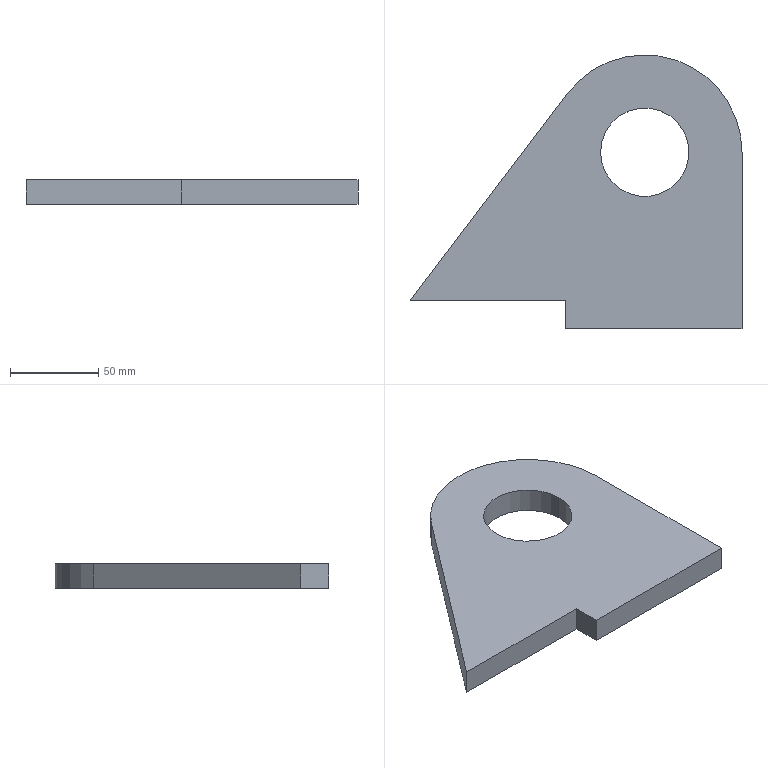Part | SolidWorks | features Extrusion 1, ICE 1 | 1 solid | 10 faces | box 187.85 x 155 x 14 mm | volume 247165 mm3 | plane 7 | cylinder 3 | commonest cylinder face diameters 50 x2 110 x1
STEP:
#1=CARTESIAN_POINT('',(-25.,0.,14.));
#2=VERTEX_POINT('',#1);
#3=CARTESIAN_POINT('',(25.,0.,14.));
#4=VERTEX_POINT('',#3);
#5=CARTESIAN_POINT('',(0.,0.,14.));
#6=DIRECTION('',(0.,0.,1.));
#7=DIRECTION('',(1.,0.,0.));
#8=AXIS2_PLACEMENT_3D('',#5,#6,#7);
#9=CIRCLE('',#8,25.);
#10=EDGE_CURVE('',#2,#4,#9,.T.);
#11=ORIENTED_EDGE('',*,*,#10,.T.);
#12=CARTESIAN_POINT('',(25.,0.,0.));
#13=VERTEX_POINT('',#12);
#14=CARTESIAN_POINT('',(25.,0.,14.));
#15=DIRECTION('',(0.,0.,-1.));
#16=VECTOR('',#15,1000.);
#17=LINE('',#14,#16);
#18=EDGE_CURVE('',#4,#13,#17,.T.);
#19=ORIENTED_EDGE('',*,*,#18,.T.);
#20=CARTESIAN_POINT('',(-25.,0.,0.));
#21=VERTEX_POINT('',#20);
#22=CARTESIAN_POINT('',(0.,0.,0.));
#23=DIRECTION('',(0.,0.,1.));
#24=DIRECTION('',(1.,0.,0.));
#25=AXIS2_PLACEMENT_3D('',#22,#23,#24);
#26=CIRCLE('',#25,25.);
#27=EDGE_CURVE('',#21,#13,#26,.T.);
#28=ORIENTED_EDGE('',*,*,#27,.F.);
#29=CARTESIAN_POINT('',(-25.,0.,14.));
#30=DIRECTION('',(0.,0.,-1.));
#31=VECTOR('',#30,1000.);
#32=LINE('',#29,#31);
#33=EDGE_CURVE('',#2,#21,#32,.T.);
#34=ORIENTED_EDGE('',*,*,#33,.F.);
#35=EDGE_LOOP('',(#11,#19,#28,#34));
#36=FACE_OUTER_BOUND('',#35,.T.);
#37=CARTESIAN_POINT('',(0.,0.,14.));
#38=DIRECTION('',(0.,0.,-1.));
#39=DIRECTION('',(-1.,0.,0.));
#40=AXIS2_PLACEMENT_3D('',#37,#38,#39);
#41=CYLINDRICAL_SURFACE('',#40,25.);
#42=ADVANCED_FACE('',(#36),#41,.F.);
#43=CARTESIAN_POINT('',(-45.,-84.,14.));
#44=VERTEX_POINT('',#43);
#45=CARTESIAN_POINT('',(-132.85,-84.,14.));
#46=VERTEX_POINT('',#45);
#47=CARTESIAN_POINT('',(-145.,-84.,14.));
#48=DIRECTION('',(-1.,0.,0.));
#49=VECTOR('',#48,1000.);
#50=LINE('',#47,#49);
#51=EDGE_CURVE('',#44,#46,#50,.T.);
#52=ORIENTED_EDGE('',*,*,#51,.F.);
#53=CARTESIAN_POINT('',(-45.,-100.,14.));
#54=VERTEX_POINT('',#53);
#55=CARTESIAN_POINT('',(-45.,-100.,14.));
#56=DIRECTION('',(0.,1.,0.));
#57=VECTOR('',#56,1000.);
#58=LINE('',#55,#57);
#59=EDGE_CURVE('',#54,#44,#58,.T.);
#60=ORIENTED_EDGE('',*,*,#59,.F.);
#61=CARTESIAN_POINT('',(55.,-100.,14.));
#62=VERTEX_POINT('',#61);
#63=CARTESIAN_POINT('',(-145.,-100.,14.));
#64=DIRECTION('',(1.,0.,0.));
#65=VECTOR('',#64,1000.);
#66=LINE('',#63,#65);
#67=EDGE_CURVE('',#54,#62,#66,.T.);
#68=ORIENTED_EDGE('',*,*,#67,.T.);
#69=CARTESIAN_POINT('',(55.,0.,14.));
#70=VERTEX_POINT('',#69);
#71=CARTESIAN_POINT('',(55.,0.,14.));
#72=DIRECTION('',(0.,1.,0.));
#73=VECTOR('',#72,1000.);
#74=LINE('',#71,#73);
#75=EDGE_CURVE('',#62,#70,#74,.T.);
#76=ORIENTED_EDGE('',*,*,#75,.T.);
#77=CARTESIAN_POINT('',(-43.802,33.263,14.));
#78=VERTEX_POINT('',#77);
#79=CARTESIAN_POINT('',(0.,0.,14.));
#80=DIRECTION('',(0.,0.,1.));
#81=DIRECTION('',(1.,0.,0.));
#82=AXIS2_PLACEMENT_3D('',#79,#80,#81);
#83=CIRCLE('',#82,55.);
#84=EDGE_CURVE('',#70,#78,#83,.T.);
#85=ORIENTED_EDGE('',*,*,#84,.T.);
#86=CARTESIAN_POINT('',(-43.802,33.263,14.));
#87=DIRECTION('',(-0.6048,-0.7964,0.));
#88=VECTOR('',#87,1000.);
#89=LINE('',#86,#88);
#90=EDGE_CURVE('',#78,#46,#89,.T.);
#91=ORIENTED_EDGE('',*,*,#90,.T.);
#92=EDGE_LOOP('',(#52,#60,#68,#76,#85,#91));
#93=FACE_OUTER_BOUND('',#92,.T.);
#94=ORIENTED_EDGE('',*,*,#10,.F.);
#95=CARTESIAN_POINT('',(0.,0.,14.));
#96=DIRECTION('',(0.,0.,1.));
#97=DIRECTION('',(1.,0.,0.));
#98=AXIS2_PLACEMENT_3D('',#95,#96,#97);
#99=CIRCLE('',#98,25.);
#100=EDGE_CURVE('',#4,#2,#99,.T.);
#101=ORIENTED_EDGE('',*,*,#100,.F.);
#102=EDGE_LOOP('',(#94,#101));
#103=FACE_BOUND('',#102,.T.);
#104=CARTESIAN_POINT('',(0.,0.,14.));
#105=DIRECTION('',(0.,0.,1.));
#106=DIRECTION('',(1.,0.,0.));
#107=AXIS2_PLACEMENT_3D('',#104,#105,#106);
#108=PLANE('',#107);
#109=ADVANCED_FACE('',(#93,#103),#108,.T.);
#110=CARTESIAN_POINT('',(-45.,-100.,0.));
#111=VERTEX_POINT('',#110);
#112=CARTESIAN_POINT('',(-45.,-84.,0.));
#113=VERTEX_POINT('',#112);
#114=CARTESIAN_POINT('',(-45.,-100.,0.));
#115=DIRECTION('',(0.,1.,0.));
#116=VECTOR('',#115,1000.);
#117=LINE('',#114,#116);
#118=EDGE_CURVE('',#111,#113,#117,.T.);
#119=ORIENTED_EDGE('',*,*,#118,.T.);
#120=CARTESIAN_POINT('',(-132.85,-84.,0.));
#121=VERTEX_POINT('',#120);
#122=CARTESIAN_POINT('',(-145.,-84.,0.));
#123=DIRECTION('',(-1.,0.,0.));
#124=VECTOR('',#123,1000.);
#125=LINE('',#122,#124);
#126=EDGE_CURVE('',#113,#121,#125,.T.);
#127=ORIENTED_EDGE('',*,*,#126,.T.);
#128=CARTESIAN_POINT('',(-43.802,33.263,0.));
#129=VERTEX_POINT('',#128);
#130=CARTESIAN_POINT('',(-43.802,33.263,0.));
#131=DIRECTION('',(-0.6048,-0.7964,0.));
#132=VECTOR('',#131,1000.);
#133=LINE('',#130,#132);
#134=EDGE_CURVE('',#129,#121,#133,.T.);
#135=ORIENTED_EDGE('',*,*,#134,.F.);
#136=CARTESIAN_POINT('',(55.,0.,0.));
#137=VERTEX_POINT('',#136);
#138=CARTESIAN_POINT('',(0.,0.,0.));
#139=DIRECTION('',(0.,0.,1.));
#140=DIRECTION('',(1.,0.,0.));
#141=AXIS2_PLACEMENT_3D('',#138,#139,#140);
#142=CIRCLE('',#141,55.);
#143=EDGE_CURVE('',#137,#129,#142,.T.);
#144=ORIENTED_EDGE('',*,*,#143,.F.);
#145=CARTESIAN_POINT('',(55.,-100.,0.));
#146=VERTEX_POINT('',#145);
#147=CARTESIAN_POINT('',(55.,0.,0.));
#148=DIRECTION('',(0.,1.,0.));
#149=VECTOR('',#148,1000.);
#150=LINE('',#147,#149);
#151=EDGE_CURVE('',#146,#137,#150,.T.);
#152=ORIENTED_EDGE('',*,*,#151,.F.);
#153=CARTESIAN_POINT('',(-145.,-100.,0.));
#154=DIRECTION('',(1.,0.,0.));
#155=VECTOR('',#154,1000.);
#156=LINE('',#153,#155);
#157=EDGE_CURVE('',#111,#146,#156,.T.);
#158=ORIENTED_EDGE('',*,*,#157,.F.);
#159=EDGE_LOOP('',(#119,#127,#135,#144,#152,#158));
#160=FACE_OUTER_BOUND('',#159,.T.);
#161=ORIENTED_EDGE('',*,*,#27,.T.);
#162=CARTESIAN_POINT('',(0.,0.,0.));
#163=DIRECTION('',(0.,0.,1.));
#164=DIRECTION('',(1.,0.,0.));
#165=AXIS2_PLACEMENT_3D('',#162,#163,#164);
#166=CIRCLE('',#165,25.);
#167=EDGE_CURVE('',#13,#21,#166,.T.);
#168=ORIENTED_EDGE('',*,*,#167,.T.);
#169=EDGE_LOOP('',(#161,#168));
#170=FACE_BOUND('',#169,.T.);
#171=CARTESIAN_POINT('',(0.,0.,0.));
#172=DIRECTION('',(0.,0.,1.));
#173=DIRECTION('',(1.,0.,0.));
#174=AXIS2_PLACEMENT_3D('',#171,#172,#173);
#175=PLANE('',#174);
#176=ADVANCED_FACE('',(#160,#170),#175,.F.);
#177=ORIENTED_EDGE('',*,*,#143,.T.);
#178=CARTESIAN_POINT('',(-43.802,33.263,14.));
#179=DIRECTION('',(0.,0.,-1.));
#180=VECTOR('',#179,1000.);
#181=LINE('',#178,#180);
#182=EDGE_CURVE('',#78,#129,#181,.T.);
#183=ORIENTED_EDGE('',*,*,#182,.F.);
#184=ORIENTED_EDGE('',*,*,#84,.F.);
#185=CARTESIAN_POINT('',(55.,0.,14.));
#186=DIRECTION('',(0.,0.,-1.));
#187=VECTOR('',#186,1000.);
#188=LINE('',#185,#187);
#189=EDGE_CURVE('',#70,#137,#188,.T.);
#190=ORIENTED_EDGE('',*,*,#189,.T.);
#191=EDGE_LOOP('',(#177,#183,#184,#190));
#192=FACE_OUTER_BOUND('',#191,.T.);
#193=CARTESIAN_POINT('',(0.,0.,14.));
#194=DIRECTION('',(0.,0.,-1.));
#195=DIRECTION('',(-1.,0.,0.));
#196=AXIS2_PLACEMENT_3D('',#193,#194,#195);
#197=CYLINDRICAL_SURFACE('',#196,55.);
#198=ADVANCED_FACE('',(#192),#197,.T.);
#199=ORIENTED_EDGE('',*,*,#134,.T.);
#200=CARTESIAN_POINT('',(-132.85,-84.,14.));
#201=DIRECTION('',(0.,0.,1.));
#202=VECTOR('',#201,1000.);
#203=LINE('',#200,#202);
#204=EDGE_CURVE('',#121,#46,#203,.T.);
#205=ORIENTED_EDGE('',*,*,#204,.T.);
#206=ORIENTED_EDGE('',*,*,#90,.F.);
#207=ORIENTED_EDGE('',*,*,#182,.T.);
#208=EDGE_LOOP('',(#199,#205,#206,#207));
#209=FACE_OUTER_BOUND('',#208,.T.);
#210=CARTESIAN_POINT('',(-43.802,33.263,14.));
#211=DIRECTION('',(0.7964,-0.6048,0.));
#212=DIRECTION('',(0.6048,0.7964,0.));
#213=AXIS2_PLACEMENT_3D('',#210,#211,#212);
#214=PLANE('',#213);
#215=ADVANCED_FACE('',(#209),#214,.F.);
#216=ORIENTED_EDGE('',*,*,#67,.F.);
#217=CARTESIAN_POINT('',(-45.,-100.,0.));
#218=DIRECTION('',(0.,0.,1.));
#219=VECTOR('',#218,1000.);
#220=LINE('',#217,#219);
#221=EDGE_CURVE('',#111,#54,#220,.T.);
#222=ORIENTED_EDGE('',*,*,#221,.F.);
#223=ORIENTED_EDGE('',*,*,#157,.T.);
#224=CARTESIAN_POINT('',(55.,-100.,14.));
#225=DIRECTION('',(0.,0.,-1.));
#226=VECTOR('',#225,1000.);
#227=LINE('',#224,#226);
#228=EDGE_CURVE('',#62,#146,#227,.T.);
#229=ORIENTED_EDGE('',*,*,#228,.F.);
#230=EDGE_LOOP('',(#216,#222,#223,#229));
#231=FACE_OUTER_BOUND('',#230,.T.);
#232=CARTESIAN_POINT('',(-145.,-100.,14.));
#233=DIRECTION('',(0.,1.,0.));
#234=DIRECTION('',(0.,0.,1.));
#235=AXIS2_PLACEMENT_3D('',#232,#233,#234);
#236=PLANE('',#235);
#237=ADVANCED_FACE('',(#231),#236,.F.);
#238=ORIENTED_EDGE('',*,*,#151,.T.);
#239=ORIENTED_EDGE('',*,*,#189,.F.);
#240=ORIENTED_EDGE('',*,*,#75,.F.);
#241=ORIENTED_EDGE('',*,*,#228,.T.);
#242=EDGE_LOOP('',(#238,#239,#240,#241));
#243=FACE_OUTER_BOUND('',#242,.T.);
#244=CARTESIAN_POINT('',(55.,0.,14.));
#245=DIRECTION('',(-1.,0.,0.));
#246=DIRECTION('',(0.,-1.,0.));
#247=AXIS2_PLACEMENT_3D('',#244,#245,#246);
#248=PLANE('',#247);
#249=ADVANCED_FACE('',(#243),#248,.F.);
#250=ORIENTED_EDGE('',*,*,#18,.F.);
#251=ORIENTED_EDGE('',*,*,#100,.T.);
#252=ORIENTED_EDGE('',*,*,#33,.T.);
#253=ORIENTED_EDGE('',*,*,#167,.F.);
#254=EDGE_LOOP('',(#250,#251,#252,#253));
#255=FACE_OUTER_BOUND('',#254,.T.);
#256=CARTESIAN_POINT('',(0.,0.,14.));
#257=DIRECTION('',(0.,0.,-1.));
#258=DIRECTION('',(-1.,0.,0.));
#259=AXIS2_PLACEMENT_3D('',#256,#257,#258);
#260=CYLINDRICAL_SURFACE('',#259,25.);
#261=ADVANCED_FACE('',(#255),#260,.F.);
#262=ORIENTED_EDGE('',*,*,#126,.F.);
#263=CARTESIAN_POINT('',(-45.,-84.,0.));
#264=DIRECTION('',(0.,0.,1.));
#265=VECTOR('',#264,1000.);
#266=LINE('',#263,#265);
#267=EDGE_CURVE('',#113,#44,#266,.T.);
#268=ORIENTED_EDGE('',*,*,#267,.T.);
#269=ORIENTED_EDGE('',*,*,#51,.T.);
#270=ORIENTED_EDGE('',*,*,#204,.F.);
#271=EDGE_LOOP('',(#262,#268,#269,#270));
#272=FACE_OUTER_BOUND('',#271,.T.);
#273=CARTESIAN_POINT('',(-145.,-84.,0.));
#274=DIRECTION('',(0.,1.,0.));
#275=DIRECTION('',(0.,0.,1.));
#276=AXIS2_PLACEMENT_3D('',#273,#274,#275);
#277=PLANE('',#276);
#278=ADVANCED_FACE('',(#272),#277,.F.);
#279=ORIENTED_EDGE('',*,*,#59,.T.);
#280=ORIENTED_EDGE('',*,*,#267,.F.);
#281=ORIENTED_EDGE('',*,*,#118,.F.);
#282=ORIENTED_EDGE('',*,*,#221,.T.);
#283=EDGE_LOOP('',(#279,#280,#281,#282));
#284=FACE_OUTER_BOUND('',#283,.T.);
#285=CARTESIAN_POINT('',(-45.,-100.,0.));
#286=DIRECTION('',(1.,0.,0.));
#287=DIRECTION('',(0.,0.,-1.));
#288=AXIS2_PLACEMENT_3D('',#285,#286,#287);
#289=PLANE('',#288);
#290=ADVANCED_FACE('',(#284),#289,.F.);
#291=CLOSED_SHELL('',(#42,#109,#176,#198,#215,#237,#249,#261,#278,#290));
#292=MANIFOLD_SOLID_BREP('',#291);
#293=CARTESIAN_POINT('',(0.,0.,0.));
#294=DIRECTION('',(0.,0.,1.));
#295=DIRECTION('',(1.,0.,0.));
#296=AXIS2_PLACEMENT_3D('',#293,#294,#295);
#297=(LENGTH_UNIT()NAMED_UNIT(*)SI_UNIT(.MILLI.,.METRE.));
#298=UNCERTAINTY_MEASURE_WITH_UNIT(LENGTH_MEASURE(0.00001),#297,'','');
#299=(NAMED_UNIT(*)PLANE_ANGLE_UNIT()SI_UNIT($,.RADIAN.));
#300=(NAMED_UNIT(*)SI_UNIT($,.STERADIAN.)SOLID_ANGLE_UNIT());
#301=(GEOMETRIC_REPRESENTATION_CONTEXT(3)GLOBAL_UNCERTAINTY_ASSIGNED_CONTEXT((#298))GLOBAL_UNIT_ASSIGNED_CONTEXT((#297,#299,#300))REPRESENTATION_CONTEXT('',''));
#302=ADVANCED_BREP_SHAPE_REPRESENTATION('',(#292,#296),#301);